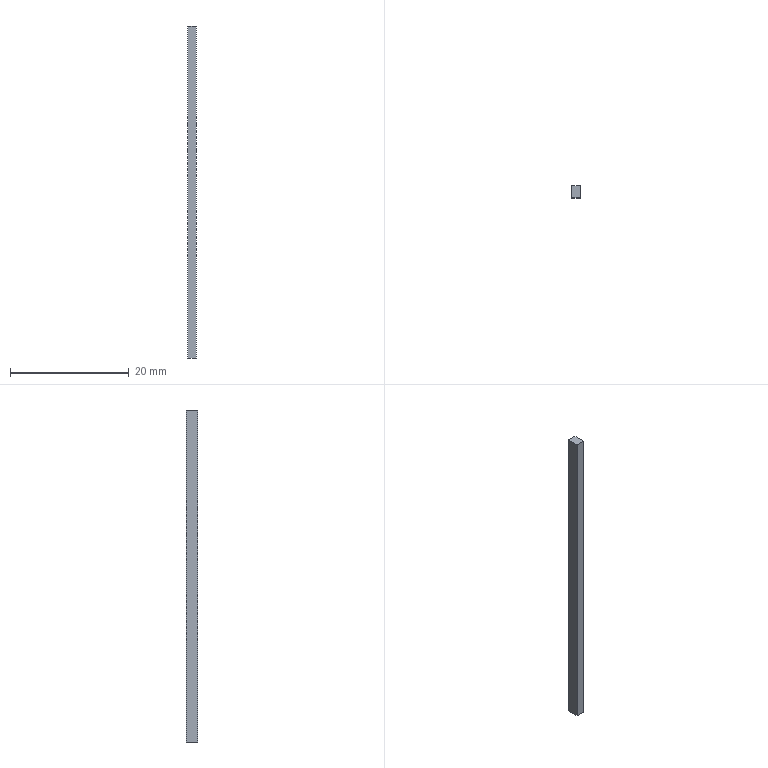Part | NX | features BREP 2 | 2 solids | 12 faces | box 1.5 x 2 x 56 mm | volume 336 mm3 | plane 12
STEP:
#1=CARTESIAN_POINT('',(0.75,-1.,-4.));
#2=VERTEX_POINT('',#1);
#3=CARTESIAN_POINT('',(0.75,-1.,52.));
#4=VERTEX_POINT('',#3);
#5=CARTESIAN_POINT('',(0.75,-1.,0.));
#6=DIRECTION('',(0.,0.,1.));
#7=VECTOR('',#6,1000.);
#8=LINE('',#5,#7);
#9=EDGE_CURVE('',#2,#4,#8,.T.);
#10=ORIENTED_EDGE('',*,*,#9,.T.);
#11=CARTESIAN_POINT('',(-0.75,-1.,52.));
#12=VERTEX_POINT('',#11);
#13=CARTESIAN_POINT('',(0.208,-1.,52.));
#14=DIRECTION('',(1.,0.,0.));
#15=VECTOR('',#14,1000.);
#16=LINE('',#13,#15);
#17=EDGE_CURVE('',#12,#4,#16,.T.);
#18=ORIENTED_EDGE('',*,*,#17,.F.);
#19=CARTESIAN_POINT('',(-0.75,-1.,-4.));
#20=VERTEX_POINT('',#19);
#21=CARTESIAN_POINT('',(-0.75,-1.,0.));
#22=DIRECTION('',(0.,0.,1.));
#23=VECTOR('',#22,1000.);
#24=LINE('',#21,#23);
#25=EDGE_CURVE('',#20,#12,#24,.T.);
#26=ORIENTED_EDGE('',*,*,#25,.F.);
#27=CARTESIAN_POINT('',(0.208,-1.,-4.));
#28=DIRECTION('',(1.,0.,0.));
#29=VECTOR('',#28,1000.);
#30=LINE('',#27,#29);
#31=EDGE_CURVE('',#20,#2,#30,.T.);
#32=ORIENTED_EDGE('',*,*,#31,.T.);
#33=EDGE_LOOP('',(#10,#18,#26,#32));
#34=FACE_BOUND('',#33,.T.);
#35=CARTESIAN_POINT('',(0.208,-1.,0.));
#36=DIRECTION('',(0.,-1.,0.));
#37=DIRECTION('',(-1.,0.,0.));
#38=AXIS2_PLACEMENT_3D('',#35,#36,#37);
#39=PLANE('',#38);
#40=ADVANCED_FACE('',(#34),#39,.T.);
#41=ORIENTED_EDGE('',*,*,#25,.T.);
#42=CARTESIAN_POINT('',(-0.75,1.,52.));
#43=VERTEX_POINT('',#42);
#44=CARTESIAN_POINT('',(-0.75,-13.298,52.));
#45=DIRECTION('',(0.,-1.,0.));
#46=VECTOR('',#45,1000.);
#47=LINE('',#44,#46);
#48=EDGE_CURVE('',#43,#12,#47,.T.);
#49=ORIENTED_EDGE('',*,*,#48,.F.);
#50=CARTESIAN_POINT('',(-0.75,1.,-4.));
#51=VERTEX_POINT('',#50);
#52=CARTESIAN_POINT('',(-0.75,1.,0.));
#53=DIRECTION('',(0.,0.,1.));
#54=VECTOR('',#53,1000.);
#55=LINE('',#52,#54);
#56=EDGE_CURVE('',#51,#43,#55,.T.);
#57=ORIENTED_EDGE('',*,*,#56,.F.);
#58=CARTESIAN_POINT('',(-0.75,-13.298,-4.));
#59=DIRECTION('',(0.,-1.,0.));
#60=VECTOR('',#59,1000.);
#61=LINE('',#58,#60);
#62=EDGE_CURVE('',#51,#20,#61,.T.);
#63=ORIENTED_EDGE('',*,*,#62,.T.);
#64=EDGE_LOOP('',(#41,#49,#57,#63));
#65=FACE_BOUND('',#64,.T.);
#66=CARTESIAN_POINT('',(-0.75,-1.493,0.));
#67=DIRECTION('',(1.,0.,0.));
#68=DIRECTION('',(0.,-1.,0.));
#69=AXIS2_PLACEMENT_3D('',#66,#67,#68);
#70=PLANE('',#69);
#71=ADVANCED_FACE('',(#65),#70,.F.);
#72=ORIENTED_EDGE('',*,*,#56,.T.);
#73=CARTESIAN_POINT('',(0.75,1.,52.));
#74=VERTEX_POINT('',#73);
#75=CARTESIAN_POINT('',(0.208,1.,52.));
#76=DIRECTION('',(-1.,0.,0.));
#77=VECTOR('',#76,1000.);
#78=LINE('',#75,#77);
#79=EDGE_CURVE('',#74,#43,#78,.T.);
#80=ORIENTED_EDGE('',*,*,#79,.F.);
#81=CARTESIAN_POINT('',(0.75,1.,-4.));
#82=VERTEX_POINT('',#81);
#83=CARTESIAN_POINT('',(0.75,1.,0.));
#84=DIRECTION('',(0.,0.,1.));
#85=VECTOR('',#84,1000.);
#86=LINE('',#83,#85);
#87=EDGE_CURVE('',#82,#74,#86,.T.);
#88=ORIENTED_EDGE('',*,*,#87,.F.);
#89=CARTESIAN_POINT('',(0.208,1.,-4.));
#90=DIRECTION('',(-1.,0.,0.));
#91=VECTOR('',#90,1000.);
#92=LINE('',#89,#91);
#93=EDGE_CURVE('',#82,#51,#92,.T.);
#94=ORIENTED_EDGE('',*,*,#93,.T.);
#95=EDGE_LOOP('',(#72,#80,#88,#94));
#96=FACE_BOUND('',#95,.T.);
#97=CARTESIAN_POINT('',(0.208,1.,0.));
#98=DIRECTION('',(0.,-1.,0.));
#99=DIRECTION('',(-1.,0.,0.));
#100=AXIS2_PLACEMENT_3D('',#97,#98,#99);
#101=PLANE('',#100);
#102=ADVANCED_FACE('',(#96),#101,.F.);
#103=CARTESIAN_POINT('',(0.75,-13.298,-4.));
#104=DIRECTION('',(0.,1.,0.));
#105=VECTOR('',#104,1000.);
#106=LINE('',#103,#105);
#107=EDGE_CURVE('',#2,#82,#106,.T.);
#108=ORIENTED_EDGE('',*,*,#107,.T.);
#109=ORIENTED_EDGE('',*,*,#87,.T.);
#110=CARTESIAN_POINT('',(0.75,-13.298,52.));
#111=DIRECTION('',(0.,1.,0.));
#112=VECTOR('',#111,1000.);
#113=LINE('',#110,#112);
#114=EDGE_CURVE('',#4,#74,#113,.T.);
#115=ORIENTED_EDGE('',*,*,#114,.F.);
#116=ORIENTED_EDGE('',*,*,#9,.F.);
#117=EDGE_LOOP('',(#108,#109,#115,#116));
#118=FACE_BOUND('',#117,.T.);
#119=CARTESIAN_POINT('',(0.75,4.,0.));
#120=DIRECTION('',(-1.,0.,0.));
#121=DIRECTION('',(0.,1.,0.));
#122=AXIS2_PLACEMENT_3D('',#119,#120,#121);
#123=PLANE('',#122);
#124=ADVANCED_FACE('',(#118),#123,.F.);
#125=ORIENTED_EDGE('',*,*,#79,.T.);
#126=ORIENTED_EDGE('',*,*,#48,.T.);
#127=ORIENTED_EDGE('',*,*,#17,.T.);
#128=ORIENTED_EDGE('',*,*,#114,.T.);
#129=EDGE_LOOP('',(#125,#126,#127,#128));
#130=FACE_BOUND('',#129,.T.);
#131=CARTESIAN_POINT('',(0.208,-13.298,52.));
#132=DIRECTION('',(0.,0.,1.));
#133=DIRECTION('',(-1.,0.,0.));
#134=AXIS2_PLACEMENT_3D('',#131,#132,#133);
#135=PLANE('',#134);
#136=ADVANCED_FACE('',(#130),#135,.T.);
#137=ORIENTED_EDGE('',*,*,#93,.F.);
#138=ORIENTED_EDGE('',*,*,#107,.F.);
#139=ORIENTED_EDGE('',*,*,#31,.F.);
#140=ORIENTED_EDGE('',*,*,#62,.F.);
#141=EDGE_LOOP('',(#137,#138,#139,#140));
#142=FACE_BOUND('',#141,.T.);
#143=CARTESIAN_POINT('',(0.208,-13.298,-4.));
#144=DIRECTION('',(0.,0.,1.));
#145=DIRECTION('',(-1.,0.,0.));
#146=AXIS2_PLACEMENT_3D('',#143,#144,#145);
#147=PLANE('',#146);
#148=ADVANCED_FACE('',(#142),#147,.F.);
#149=CLOSED_SHELL('',(#40,#71,#102,#124,#136,#148));
#150=MANIFOLD_SOLID_BREP('',#149);
#151=CARTESIAN_POINT('',(0.75,-1.,-4.));
#152=VERTEX_POINT('',#151);
#153=CARTESIAN_POINT('',(0.75,-1.,52.));
#154=VERTEX_POINT('',#153);
#155=CARTESIAN_POINT('',(0.75,-1.,0.));
#156=DIRECTION('',(0.,0.,1.));
#157=VECTOR('',#156,1000.);
#158=LINE('',#155,#157);
#159=EDGE_CURVE('',#152,#154,#158,.T.);
#160=ORIENTED_EDGE('',*,*,#159,.T.);
#161=CARTESIAN_POINT('',(-0.75,-1.,52.));
#162=VERTEX_POINT('',#161);
#163=CARTESIAN_POINT('',(0.208,-1.,52.));
#164=DIRECTION('',(1.,0.,0.));
#165=VECTOR('',#164,1000.);
#166=LINE('',#163,#165);
#167=EDGE_CURVE('',#162,#154,#166,.T.);
#168=ORIENTED_EDGE('',*,*,#167,.F.);
#169=CARTESIAN_POINT('',(-0.75,-1.,-4.));
#170=VERTEX_POINT('',#169);
#171=CARTESIAN_POINT('',(-0.75,-1.,0.));
#172=DIRECTION('',(0.,0.,1.));
#173=VECTOR('',#172,1000.);
#174=LINE('',#171,#173);
#175=EDGE_CURVE('',#170,#162,#174,.T.);
#176=ORIENTED_EDGE('',*,*,#175,.F.);
#177=CARTESIAN_POINT('',(0.208,-1.,-4.));
#178=DIRECTION('',(1.,0.,0.));
#179=VECTOR('',#178,1000.);
#180=LINE('',#177,#179);
#181=EDGE_CURVE('',#170,#152,#180,.T.);
#182=ORIENTED_EDGE('',*,*,#181,.T.);
#183=EDGE_LOOP('',(#160,#168,#176,#182));
#184=FACE_BOUND('',#183,.T.);
#185=CARTESIAN_POINT('',(0.208,-1.,0.));
#186=DIRECTION('',(0.,-1.,0.));
#187=DIRECTION('',(-1.,0.,0.));
#188=AXIS2_PLACEMENT_3D('',#185,#186,#187);
#189=PLANE('',#188);
#190=ADVANCED_FACE('',(#184),#189,.T.);
#191=ORIENTED_EDGE('',*,*,#175,.T.);
#192=CARTESIAN_POINT('',(-0.75,1.,52.));
#193=VERTEX_POINT('',#192);
#194=CARTESIAN_POINT('',(-0.75,-13.298,52.));
#195=DIRECTION('',(0.,-1.,0.));
#196=VECTOR('',#195,1000.);
#197=LINE('',#194,#196);
#198=EDGE_CURVE('',#193,#162,#197,.T.);
#199=ORIENTED_EDGE('',*,*,#198,.F.);
#200=CARTESIAN_POINT('',(-0.75,1.,-4.));
#201=VERTEX_POINT('',#200);
#202=CARTESIAN_POINT('',(-0.75,1.,0.));
#203=DIRECTION('',(0.,0.,1.));
#204=VECTOR('',#203,1000.);
#205=LINE('',#202,#204);
#206=EDGE_CURVE('',#201,#193,#205,.T.);
#207=ORIENTED_EDGE('',*,*,#206,.F.);
#208=CARTESIAN_POINT('',(-0.75,-13.298,-4.));
#209=DIRECTION('',(0.,-1.,0.));
#210=VECTOR('',#209,1000.);
#211=LINE('',#208,#210);
#212=EDGE_CURVE('',#201,#170,#211,.T.);
#213=ORIENTED_EDGE('',*,*,#212,.T.);
#214=EDGE_LOOP('',(#191,#199,#207,#213));
#215=FACE_BOUND('',#214,.T.);
#216=CARTESIAN_POINT('',(-0.75,-1.493,0.));
#217=DIRECTION('',(1.,0.,0.));
#218=DIRECTION('',(0.,-1.,0.));
#219=AXIS2_PLACEMENT_3D('',#216,#217,#218);
#220=PLANE('',#219);
#221=ADVANCED_FACE('',(#215),#220,.F.);
#222=ORIENTED_EDGE('',*,*,#206,.T.);
#223=CARTESIAN_POINT('',(0.75,1.,52.));
#224=VERTEX_POINT('',#223);
#225=CARTESIAN_POINT('',(0.208,1.,52.));
#226=DIRECTION('',(-1.,0.,0.));
#227=VECTOR('',#226,1000.);
#228=LINE('',#225,#227);
#229=EDGE_CURVE('',#224,#193,#228,.T.);
#230=ORIENTED_EDGE('',*,*,#229,.F.);
#231=CARTESIAN_POINT('',(0.75,1.,-4.));
#232=VERTEX_POINT('',#231);
#233=CARTESIAN_POINT('',(0.75,1.,0.));
#234=DIRECTION('',(0.,0.,1.));
#235=VECTOR('',#234,1000.);
#236=LINE('',#233,#235);
#237=EDGE_CURVE('',#232,#224,#236,.T.);
#238=ORIENTED_EDGE('',*,*,#237,.F.);
#239=CARTESIAN_POINT('',(0.208,1.,-4.));
#240=DIRECTION('',(-1.,0.,0.));
#241=VECTOR('',#240,1000.);
#242=LINE('',#239,#241);
#243=EDGE_CURVE('',#232,#201,#242,.T.);
#244=ORIENTED_EDGE('',*,*,#243,.T.);
#245=EDGE_LOOP('',(#222,#230,#238,#244));
#246=FACE_BOUND('',#245,.T.);
#247=CARTESIAN_POINT('',(0.208,1.,0.));
#248=DIRECTION('',(0.,-1.,0.));
#249=DIRECTION('',(-1.,0.,0.));
#250=AXIS2_PLACEMENT_3D('',#247,#248,#249);
#251=PLANE('',#250);
#252=ADVANCED_FACE('',(#246),#251,.F.);
#253=CARTESIAN_POINT('',(0.75,-13.298,-4.));
#254=DIRECTION('',(0.,1.,0.));
#255=VECTOR('',#254,1000.);
#256=LINE('',#253,#255);
#257=EDGE_CURVE('',#152,#232,#256,.T.);
#258=ORIENTED_EDGE('',*,*,#257,.T.);
#259=ORIENTED_EDGE('',*,*,#237,.T.);
#260=CARTESIAN_POINT('',(0.75,-13.298,52.));
#261=DIRECTION('',(0.,1.,0.));
#262=VECTOR('',#261,1000.);
#263=LINE('',#260,#262);
#264=EDGE_CURVE('',#154,#224,#263,.T.);
#265=ORIENTED_EDGE('',*,*,#264,.F.);
#266=ORIENTED_EDGE('',*,*,#159,.F.);
#267=EDGE_LOOP('',(#258,#259,#265,#266));
#268=FACE_BOUND('',#267,.T.);
#269=CARTESIAN_POINT('',(0.75,4.,0.));
#270=DIRECTION('',(-1.,0.,0.));
#271=DIRECTION('',(0.,1.,0.));
#272=AXIS2_PLACEMENT_3D('',#269,#270,#271);
#273=PLANE('',#272);
#274=ADVANCED_FACE('',(#268),#273,.F.);
#275=ORIENTED_EDGE('',*,*,#229,.T.);
#276=ORIENTED_EDGE('',*,*,#198,.T.);
#277=ORIENTED_EDGE('',*,*,#167,.T.);
#278=ORIENTED_EDGE('',*,*,#264,.T.);
#279=EDGE_LOOP('',(#275,#276,#277,#278));
#280=FACE_BOUND('',#279,.T.);
#281=CARTESIAN_POINT('',(0.208,-13.298,52.));
#282=DIRECTION('',(0.,0.,1.));
#283=DIRECTION('',(-1.,0.,0.));
#284=AXIS2_PLACEMENT_3D('',#281,#282,#283);
#285=PLANE('',#284);
#286=ADVANCED_FACE('',(#280),#285,.T.);
#287=ORIENTED_EDGE('',*,*,#243,.F.);
#288=ORIENTED_EDGE('',*,*,#257,.F.);
#289=ORIENTED_EDGE('',*,*,#181,.F.);
#290=ORIENTED_EDGE('',*,*,#212,.F.);
#291=EDGE_LOOP('',(#287,#288,#289,#290));
#292=FACE_BOUND('',#291,.T.);
#293=CARTESIAN_POINT('',(0.208,-13.298,-4.));
#294=DIRECTION('',(0.,0.,1.));
#295=DIRECTION('',(-1.,0.,0.));
#296=AXIS2_PLACEMENT_3D('',#293,#294,#295);
#297=PLANE('',#296);
#298=ADVANCED_FACE('',(#292),#297,.F.);
#299=CLOSED_SHELL('',(#190,#221,#252,#274,#286,#298));
#300=MANIFOLD_SOLID_BREP('',#299);
#301=(LENGTH_UNIT()NAMED_UNIT(*)SI_UNIT(.MILLI.,.METRE.));
#302=UNCERTAINTY_MEASURE_WITH_UNIT(LENGTH_MEASURE(0.00001),#301,'','');
#303=(NAMED_UNIT(*)PLANE_ANGLE_UNIT()SI_UNIT($,.RADIAN.));
#304=(NAMED_UNIT(*)SI_UNIT($,.STERADIAN.)SOLID_ANGLE_UNIT());
#305=(GEOMETRIC_REPRESENTATION_CONTEXT(3)GLOBAL_UNCERTAINTY_ASSIGNED_CONTEXT((#302))GLOBAL_UNIT_ASSIGNED_CONTEXT((#301,#303,#304))REPRESENTATION_CONTEXT('',''));
#306=ADVANCED_BREP_SHAPE_REPRESENTATION('',(#150,#300),#305);